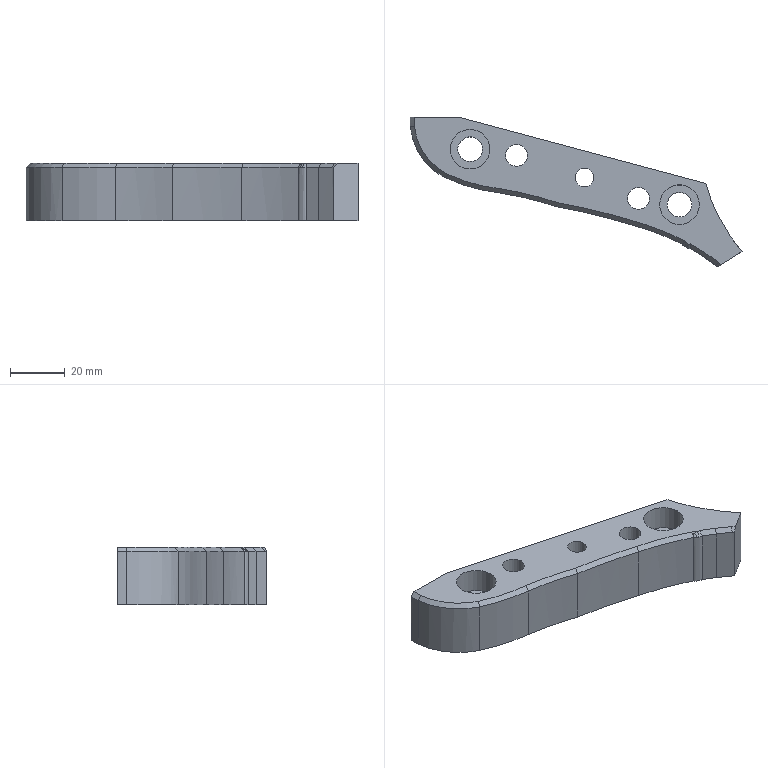Part | NX | features 23 2 | 1 solid | 37 faces | box 121.336 x 54.717 x 21 mm | volume 47317 mm3 | spline 12 | plane 10 | cone 8 | cylinder 7 | commonest cylinder face diameters 8.001 x2 9 x2 14.5 x2 6.8 x1